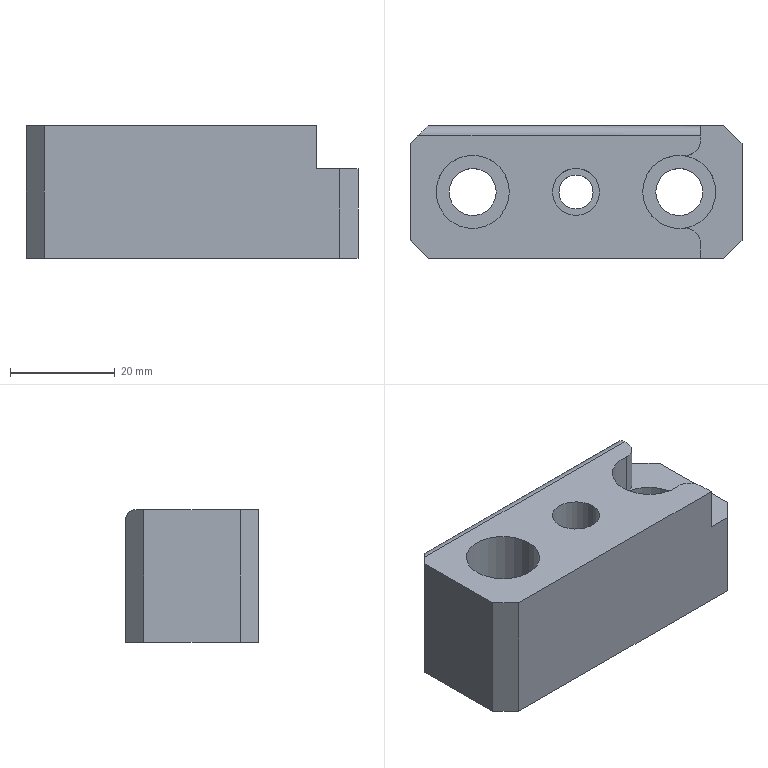Part | STEP file | 1_id1522_x_t | 1 solid | 31 faces | box 63.5 x 25.4 x 25.4 mm | volume 31340 mm3 | plane 16 | cylinder 15 | commonest cylinder face diameters 9 x6 14 x4 6 x2 6.528 x2 4 x1